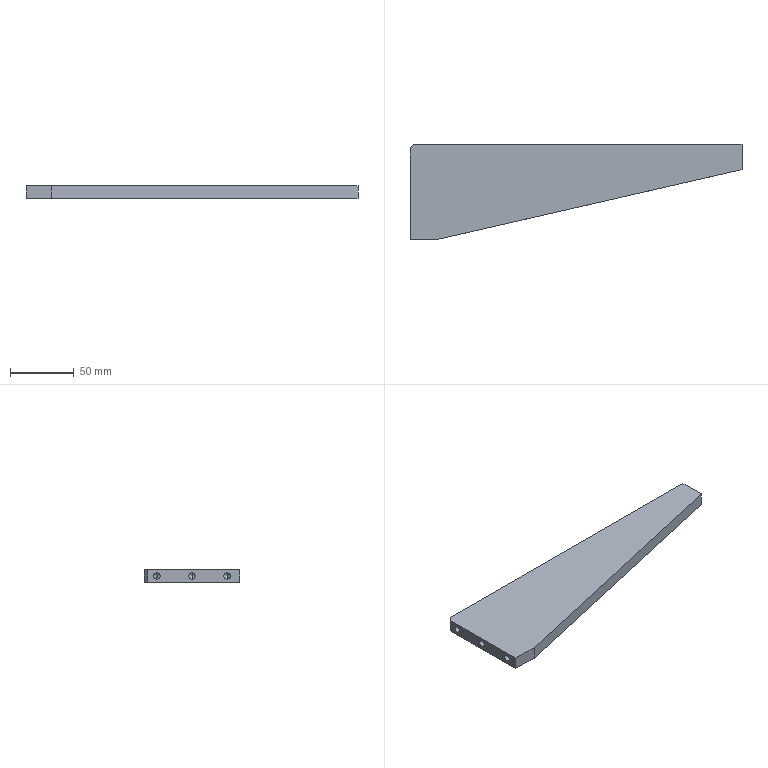Part | STEP file | PN_0009 | 1 solid | 32 faces | box 260 x 75 x 10 mm | volume 127129 mm3 | cylinder 12 | cone 12 | plane 8 | commonest cylinder face diameters 5 x12